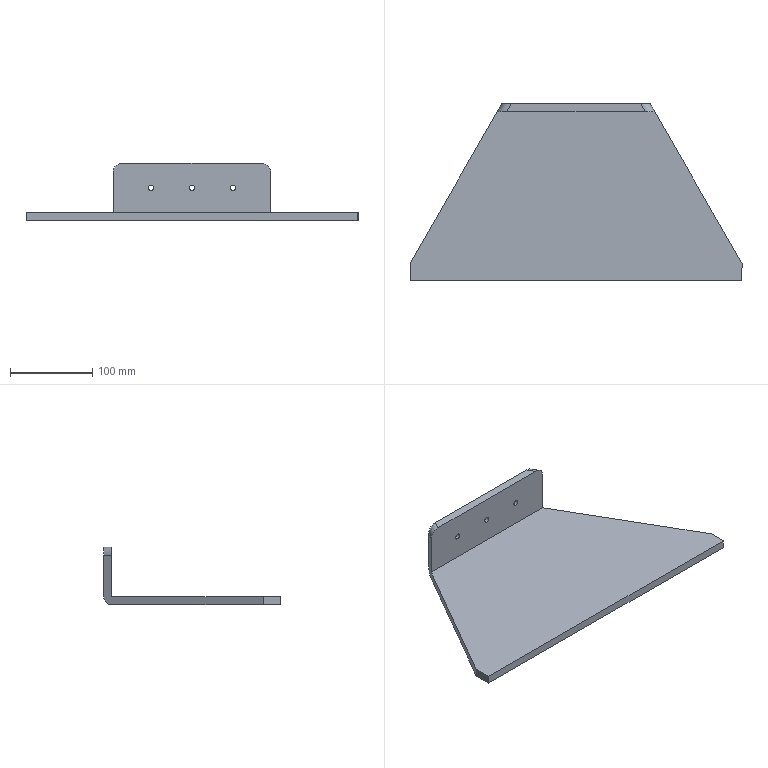Part | SolidWorks | features ICE 2, Extrusion 1, Fillet 1, HoleWzd 1, Shell 1 | 1 solid | 19 faces | box 404 x 215 x 70 mm | volume 757292 mm3 | plane 10 | cylinder 9 | commonest cylinder face diameters 6.8 x6 20 x3
STEP:
#1=CARTESIAN_POINT('',(-50.,97.5,43.4));
#2=VERTEX_POINT('',#1);
#3=CARTESIAN_POINT('',(-50.,97.5,36.6));
#4=VERTEX_POINT('',#3);
#5=CARTESIAN_POINT('',(-50.,97.5,40.));
#6=DIRECTION('',(0.,-1.,0.));
#7=DIRECTION('',(0.,0.,-1.));
#8=AXIS2_PLACEMENT_3D('',#5,#6,#7);
#9=CIRCLE('',#8,3.4);
#10=EDGE_CURVE('',#2,#4,#9,.T.);
#11=ORIENTED_EDGE('',*,*,#10,.T.);
#12=CARTESIAN_POINT('',(-50.,107.5,36.6));
#13=VERTEX_POINT('',#12);
#14=CARTESIAN_POINT('',(-50.,107.5,36.6));
#15=DIRECTION('',(0.,1.,0.));
#16=VECTOR('',#15,1000.);
#17=LINE('',#14,#16);
#18=EDGE_CURVE('',#4,#13,#17,.T.);
#19=ORIENTED_EDGE('',*,*,#18,.T.);
#20=CARTESIAN_POINT('',(-50.,107.5,43.4));
#21=VERTEX_POINT('',#20);
#22=CARTESIAN_POINT('',(-50.,107.5,40.));
#23=DIRECTION('',(0.,1.,0.));
#24=DIRECTION('',(0.,0.,1.));
#25=AXIS2_PLACEMENT_3D('',#22,#23,#24);
#26=CIRCLE('',#25,3.4);
#27=EDGE_CURVE('',#13,#21,#26,.T.);
#28=ORIENTED_EDGE('',*,*,#27,.T.);
#29=CARTESIAN_POINT('',(-50.,107.5,43.4));
#30=DIRECTION('',(0.,1.,0.));
#31=VECTOR('',#30,1000.);
#32=LINE('',#29,#31);
#33=EDGE_CURVE('',#2,#21,#32,.T.);
#34=ORIENTED_EDGE('',*,*,#33,.F.);
#35=EDGE_LOOP('',(#11,#19,#28,#34));
#36=FACE_OUTER_BOUND('',#35,.T.);
#37=CARTESIAN_POINT('',(-50.,107.5,40.));
#38=DIRECTION('',(0.,1.,0.));
#39=DIRECTION('',(0.,0.,1.));
#40=AXIS2_PLACEMENT_3D('',#37,#38,#39);
#41=CYLINDRICAL_SURFACE('',#40,3.4);
#42=ADVANCED_FACE('',(#36),#41,.F.);
#43=CARTESIAN_POINT('',(0.,97.5,43.4));
#44=VERTEX_POINT('',#43);
#45=CARTESIAN_POINT('',(0.,97.5,36.6));
#46=VERTEX_POINT('',#45);
#47=CARTESIAN_POINT('',(0.,97.5,40.));
#48=DIRECTION('',(0.,-1.,0.));
#49=DIRECTION('',(0.,0.,-1.));
#50=AXIS2_PLACEMENT_3D('',#47,#48,#49);
#51=CIRCLE('',#50,3.4);
#52=EDGE_CURVE('',#44,#46,#51,.T.);
#53=ORIENTED_EDGE('',*,*,#52,.T.);
#54=CARTESIAN_POINT('',(0.,107.5,36.6));
#55=VERTEX_POINT('',#54);
#56=CARTESIAN_POINT('',(0.,107.5,36.6));
#57=DIRECTION('',(0.,1.,0.));
#58=VECTOR('',#57,1000.);
#59=LINE('',#56,#58);
#60=EDGE_CURVE('',#46,#55,#59,.T.);
#61=ORIENTED_EDGE('',*,*,#60,.T.);
#62=CARTESIAN_POINT('',(0.,107.5,43.4));
#63=VERTEX_POINT('',#62);
#64=CARTESIAN_POINT('',(0.,107.5,40.));
#65=DIRECTION('',(0.,1.,0.));
#66=DIRECTION('',(0.,0.,1.));
#67=AXIS2_PLACEMENT_3D('',#64,#65,#66);
#68=CIRCLE('',#67,3.4);
#69=EDGE_CURVE('',#55,#63,#68,.T.);
#70=ORIENTED_EDGE('',*,*,#69,.T.);
#71=CARTESIAN_POINT('',(0.,107.5,43.4));
#72=DIRECTION('',(0.,1.,0.));
#73=VECTOR('',#72,1000.);
#74=LINE('',#71,#73);
#75=EDGE_CURVE('',#44,#63,#74,.T.);
#76=ORIENTED_EDGE('',*,*,#75,.F.);
#77=EDGE_LOOP('',(#53,#61,#70,#76));
#78=FACE_OUTER_BOUND('',#77,.T.);
#79=CARTESIAN_POINT('',(0.,107.5,40.));
#80=DIRECTION('',(0.,1.,0.));
#81=DIRECTION('',(0.,0.,1.));
#82=AXIS2_PLACEMENT_3D('',#79,#80,#81);
#83=CYLINDRICAL_SURFACE('',#82,3.4);
#84=ADVANCED_FACE('',(#78),#83,.F.);
#85=CARTESIAN_POINT('',(50.,97.5,43.4));
#86=VERTEX_POINT('',#85);
#87=CARTESIAN_POINT('',(50.,97.5,36.6));
#88=VERTEX_POINT('',#87);
#89=CARTESIAN_POINT('',(50.,97.5,40.));
#90=DIRECTION('',(0.,-1.,0.));
#91=DIRECTION('',(0.,0.,-1.));
#92=AXIS2_PLACEMENT_3D('',#89,#90,#91);
#93=CIRCLE('',#92,3.4);
#94=EDGE_CURVE('',#86,#88,#93,.T.);
#95=ORIENTED_EDGE('',*,*,#94,.T.);
#96=CARTESIAN_POINT('',(50.,107.5,36.6));
#97=VERTEX_POINT('',#96);
#98=CARTESIAN_POINT('',(50.,107.5,36.6));
#99=DIRECTION('',(0.,1.,0.));
#100=VECTOR('',#99,1000.);
#101=LINE('',#98,#100);
#102=EDGE_CURVE('',#88,#97,#101,.T.);
#103=ORIENTED_EDGE('',*,*,#102,.T.);
#104=CARTESIAN_POINT('',(50.,107.5,43.4));
#105=VERTEX_POINT('',#104);
#106=CARTESIAN_POINT('',(50.,107.5,40.));
#107=DIRECTION('',(0.,1.,0.));
#108=DIRECTION('',(0.,0.,1.));
#109=AXIS2_PLACEMENT_3D('',#106,#107,#108);
#110=CIRCLE('',#109,3.4);
#111=EDGE_CURVE('',#97,#105,#110,.T.);
#112=ORIENTED_EDGE('',*,*,#111,.T.);
#113=CARTESIAN_POINT('',(50.,107.5,43.4));
#114=DIRECTION('',(0.,1.,0.));
#115=VECTOR('',#114,1000.);
#116=LINE('',#113,#115);
#117=EDGE_CURVE('',#86,#105,#116,.T.);
#118=ORIENTED_EDGE('',*,*,#117,.F.);
#119=EDGE_LOOP('',(#95,#103,#112,#118));
#120=FACE_OUTER_BOUND('',#119,.T.);
#121=CARTESIAN_POINT('',(50.,107.5,40.));
#122=DIRECTION('',(0.,1.,0.));
#123=DIRECTION('',(0.,0.,1.));
#124=AXIS2_PLACEMENT_3D('',#121,#122,#123);
#125=CYLINDRICAL_SURFACE('',#124,3.4);
#126=ADVANCED_FACE('',(#120),#125,.F.);
#127=CARTESIAN_POINT('',(202.,-107.5,10.));
#128=VERTEX_POINT('',#127);
#129=CARTESIAN_POINT('',(202.,-86.49,10.));
#130=VERTEX_POINT('',#129);
#131=CARTESIAN_POINT('',(202.,107.5,10.));
#132=DIRECTION('',(0.,1.,0.));
#133=VECTOR('',#132,1000.);
#134=LINE('',#131,#133);
#135=EDGE_CURVE('',#128,#130,#134,.T.);
#136=ORIENTED_EDGE('',*,*,#135,.F.);
#137=CARTESIAN_POINT('',(202.,-107.5,0.));
#138=VERTEX_POINT('',#137);
#139=CARTESIAN_POINT('',(202.,-107.5,70.));
#140=DIRECTION('',(0.,0.,-1.));
#141=VECTOR('',#140,1000.);
#142=LINE('',#139,#141);
#143=EDGE_CURVE('',#128,#138,#142,.T.);
#144=ORIENTED_EDGE('',*,*,#143,.T.);
#145=CARTESIAN_POINT('',(202.,-86.49,0.));
#146=VERTEX_POINT('',#145);
#147=CARTESIAN_POINT('',(202.,107.5,0.));
#148=DIRECTION('',(0.,1.,0.));
#149=VECTOR('',#148,1000.);
#150=LINE('',#147,#149);
#151=EDGE_CURVE('',#138,#146,#150,.T.);
#152=ORIENTED_EDGE('',*,*,#151,.T.);
#153=CARTESIAN_POINT('',(202.,-86.49,-10.));
#154=DIRECTION('',(0.,0.,1.));
#155=VECTOR('',#154,1000.);
#156=LINE('',#153,#155);
#157=EDGE_CURVE('',#146,#130,#156,.T.);
#158=ORIENTED_EDGE('',*,*,#157,.T.);
#159=EDGE_LOOP('',(#136,#144,#152,#158));
#160=FACE_OUTER_BOUND('',#159,.T.);
#161=CARTESIAN_POINT('',(202.,107.5,70.));
#162=DIRECTION('',(-1.,0.,0.));
#163=DIRECTION('',(0.,-1.,0.));
#164=AXIS2_PLACEMENT_3D('',#161,#162,#163);
#165=PLANE('',#164);
#166=ADVANCED_FACE('',(#160),#165,.F.);
#167=CARTESIAN_POINT('',(-202.,-107.5,10.));
#168=VERTEX_POINT('',#167);
#169=CARTESIAN_POINT('',(-202.,-107.5,0.));
#170=VERTEX_POINT('',#169);
#171=CARTESIAN_POINT('',(-202.,-107.5,70.));
#172=DIRECTION('',(0.,0.,-1.));
#173=VECTOR('',#172,1000.);
#174=LINE('',#171,#173);
#175=EDGE_CURVE('',#168,#170,#174,.T.);
#176=ORIENTED_EDGE('',*,*,#175,.F.);
#177=CARTESIAN_POINT('',(-202.,-86.49,10.));
#178=VERTEX_POINT('',#177);
#179=CARTESIAN_POINT('',(-202.,107.5,10.));
#180=DIRECTION('',(0.,-1.,0.));
#181=VECTOR('',#180,1000.);
#182=LINE('',#179,#181);
#183=EDGE_CURVE('',#178,#168,#182,.T.);
#184=ORIENTED_EDGE('',*,*,#183,.F.);
#185=CARTESIAN_POINT('',(-202.,-86.49,0.));
#186=VERTEX_POINT('',#185);
#187=CARTESIAN_POINT('',(-202.,-86.49,-10.));
#188=DIRECTION('',(0.,0.,1.));
#189=VECTOR('',#188,1000.);
#190=LINE('',#187,#189);
#191=EDGE_CURVE('',#186,#178,#190,.T.);
#192=ORIENTED_EDGE('',*,*,#191,.F.);
#193=CARTESIAN_POINT('',(-202.,107.5,0.));
#194=DIRECTION('',(0.,-1.,0.));
#195=VECTOR('',#194,1000.);
#196=LINE('',#193,#195);
#197=EDGE_CURVE('',#186,#170,#196,.T.);
#198=ORIENTED_EDGE('',*,*,#197,.T.);
#199=EDGE_LOOP('',(#176,#184,#192,#198));
#200=FACE_OUTER_BOUND('',#199,.T.);
#201=CARTESIAN_POINT('',(-202.,107.5,70.));
#202=DIRECTION('',(1.,0.,0.));
#203=DIRECTION('',(0.,0.,-1.));
#204=AXIS2_PLACEMENT_3D('',#201,#202,#203);
#205=PLANE('',#204);
#206=ADVANCED_FACE('',(#200),#205,.F.);
#207=CARTESIAN_POINT('',(-50.,107.5,40.));
#208=DIRECTION('',(0.,1.,0.));
#209=DIRECTION('',(0.,0.,1.));
#210=AXIS2_PLACEMENT_3D('',#207,#208,#209);
#211=CIRCLE('',#210,3.4);
#212=EDGE_CURVE('',#21,#13,#211,.T.);
#213=ORIENTED_EDGE('',*,*,#212,.F.);
#214=ORIENTED_EDGE('',*,*,#27,.F.);
#215=EDGE_LOOP('',(#213,#214));
#216=FACE_BOUND('',#215,.T.);
#217=CARTESIAN_POINT('',(0.,107.5,40.));
#218=DIRECTION('',(0.,1.,0.));
#219=DIRECTION('',(0.,0.,1.));
#220=AXIS2_PLACEMENT_3D('',#217,#218,#219);
#221=CIRCLE('',#220,3.4);
#222=EDGE_CURVE('',#63,#55,#221,.T.);
#223=ORIENTED_EDGE('',*,*,#222,.F.);
#224=ORIENTED_EDGE('',*,*,#69,.F.);
#225=EDGE_LOOP('',(#223,#224));
#226=FACE_BOUND('',#225,.T.);
#227=CARTESIAN_POINT('',(50.,107.5,40.));
#228=DIRECTION('',(0.,1.,0.));
#229=DIRECTION('',(0.,0.,1.));
#230=AXIS2_PLACEMENT_3D('',#227,#228,#229);
#231=CIRCLE('',#230,3.4);
#232=EDGE_CURVE('',#105,#97,#231,.T.);
#233=ORIENTED_EDGE('',*,*,#232,.F.);
#234=ORIENTED_EDGE('',*,*,#111,.F.);
#235=EDGE_LOOP('',(#233,#234));
#236=FACE_BOUND('',#235,.T.);
#237=CARTESIAN_POINT('',(90.,107.5,10.));
#238=VERTEX_POINT('',#237);
#239=CARTESIAN_POINT('',(90.,107.5,60.));
#240=VERTEX_POINT('',#239);
#241=CARTESIAN_POINT('',(90.,107.5,-10.));
#242=DIRECTION('',(0.,0.,1.));
#243=VECTOR('',#242,1000.);
#244=LINE('',#241,#243);
#245=EDGE_CURVE('',#238,#240,#244,.T.);
#246=ORIENTED_EDGE('',*,*,#245,.F.);
#247=CARTESIAN_POINT('',(-90.,107.5,10.));
#248=VERTEX_POINT('',#247);
#249=CARTESIAN_POINT('',(-202.,107.5,10.));
#250=DIRECTION('',(-1.,0.,0.));
#251=VECTOR('',#250,1000.);
#252=LINE('',#249,#251);
#253=EDGE_CURVE('',#238,#248,#252,.T.);
#254=ORIENTED_EDGE('',*,*,#253,.T.);
#255=CARTESIAN_POINT('',(-90.,107.5,60.));
#256=VERTEX_POINT('',#255);
#257=CARTESIAN_POINT('',(-90.,107.5,-10.));
#258=DIRECTION('',(0.,0.,1.));
#259=VECTOR('',#258,1000.);
#260=LINE('',#257,#259);
#261=EDGE_CURVE('',#248,#256,#260,.T.);
#262=ORIENTED_EDGE('',*,*,#261,.T.);
#263=CARTESIAN_POINT('',(-78.453,107.5,70.));
#264=VERTEX_POINT('',#263);
#265=CARTESIAN_POINT('',(-90.,107.5,60.));
#266=CARTESIAN_POINT('',(-90.,107.5,65.858));
#267=CARTESIAN_POINT('',(-85.217,107.5,70.));
#268=CARTESIAN_POINT('',(-78.453,107.5,70.));
#269=(BOUNDED_CURVE()B_SPLINE_CURVE(3,(#265,#266,#267,#268),.UNSPECIFIED.,.F.,.F.)B_SPLINE_CURVE_WITH_KNOTS((4,4),(0.,1.571),.UNSPECIFIED.)CURVE()GEOMETRIC_REPRESENTATION_ITEM()RATIONAL_B_SPLINE_CURVE((1.,0.8047,0.8047,1.))REPRESENTATION_ITEM(''));
#270=EDGE_CURVE('',#256,#264,#269,.T.);
#271=ORIENTED_EDGE('',*,*,#270,.T.);
#272=CARTESIAN_POINT('',(78.453,107.5,70.));
#273=VERTEX_POINT('',#272);
#274=CARTESIAN_POINT('',(-202.,107.5,70.));
#275=DIRECTION('',(-1.,0.,0.));
#276=VECTOR('',#275,1000.);
#277=LINE('',#274,#276);
#278=EDGE_CURVE('',#273,#264,#277,.T.);
#279=ORIENTED_EDGE('',*,*,#278,.F.);
#280=CARTESIAN_POINT('',(78.453,107.5,70.));
#281=CARTESIAN_POINT('',(85.217,107.5,70.));
#282=CARTESIAN_POINT('',(90.,107.5,65.858));
#283=CARTESIAN_POINT('',(90.,107.5,60.));
#284=(BOUNDED_CURVE()B_SPLINE_CURVE(3,(#280,#281,#282,#283),.UNSPECIFIED.,.F.,.F.)B_SPLINE_CURVE_WITH_KNOTS((4,4),(1.571,3.142),.UNSPECIFIED.)CURVE()GEOMETRIC_REPRESENTATION_ITEM()RATIONAL_B_SPLINE_CURVE((1.,0.8047,0.8047,1.))REPRESENTATION_ITEM(''));
#285=EDGE_CURVE('',#273,#240,#284,.T.);
#286=ORIENTED_EDGE('',*,*,#285,.T.);
#287=EDGE_LOOP('',(#246,#254,#262,#271,#279,#286));
#288=FACE_OUTER_BOUND('',#287,.T.);
#289=CARTESIAN_POINT('',(-202.,107.5,70.));
#290=DIRECTION('',(0.,-1.,0.));
#291=DIRECTION('',(0.,0.,-1.));
#292=AXIS2_PLACEMENT_3D('',#289,#290,#291);
#293=PLANE('',#292);
#294=ADVANCED_FACE('',(#216,#226,#236,#288),#293,.F.);
#295=ORIENTED_EDGE('',*,*,#143,.F.);
#296=CARTESIAN_POINT('',(-642.963,-107.5,10.));
#297=DIRECTION('',(1.,0.,0.));
#298=VECTOR('',#297,1000.);
#299=LINE('',#296,#298);
#300=EDGE_CURVE('',#168,#128,#299,.T.);
#301=ORIENTED_EDGE('',*,*,#300,.F.);
#302=ORIENTED_EDGE('',*,*,#175,.T.);
#303=CARTESIAN_POINT('',(-202.,-107.5,0.));
#304=DIRECTION('',(1.,0.,0.));
#305=VECTOR('',#304,1000.);
#306=LINE('',#303,#305);
#307=EDGE_CURVE('',#170,#138,#306,.T.);
#308=ORIENTED_EDGE('',*,*,#307,.T.);
#309=EDGE_LOOP('',(#295,#301,#302,#308));
#310=FACE_OUTER_BOUND('',#309,.T.);
#311=CARTESIAN_POINT('',(-202.,-107.5,70.));
#312=DIRECTION('',(0.,1.,0.));
#313=DIRECTION('',(0.,0.,1.));
#314=AXIS2_PLACEMENT_3D('',#311,#312,#313);
#315=PLANE('',#314);
#316=ADVANCED_FACE('',(#310),#315,.F.);
#317=CARTESIAN_POINT('',(84.226,97.5,70.));
#318=VERTEX_POINT('',#317);
#319=CARTESIAN_POINT('',(-84.226,97.5,70.));
#320=VERTEX_POINT('',#319);
#321=CARTESIAN_POINT('',(0.,97.5,70.));
#322=DIRECTION('',(-1.,0.,0.));
#323=VECTOR('',#322,1000.);
#324=LINE('',#321,#323);
#325=EDGE_CURVE('',#318,#320,#324,.T.);
#326=ORIENTED_EDGE('',*,*,#325,.F.);
#327=CARTESIAN_POINT('',(81.34,102.5,70.));
#328=DIRECTION('',(-0.5,0.866,0.));
#329=VECTOR('',#328,1000.);
#330=LINE('',#327,#329);
#331=EDGE_CURVE('',#318,#273,#330,.T.);
#332=ORIENTED_EDGE('',*,*,#331,.T.);
#333=ORIENTED_EDGE('',*,*,#278,.T.);
#334=CARTESIAN_POINT('',(-87.113,92.5,70.));
#335=DIRECTION('',(-0.5,-0.866,0.));
#336=VECTOR('',#335,1000.);
#337=LINE('',#334,#336);
#338=EDGE_CURVE('',#264,#320,#337,.T.);
#339=ORIENTED_EDGE('',*,*,#338,.T.);
#340=EDGE_LOOP('',(#326,#332,#333,#339));
#341=FACE_OUTER_BOUND('',#340,.T.);
#342=CARTESIAN_POINT('',(0.,0.,70.));
#343=DIRECTION('',(0.,0.,1.));
#344=DIRECTION('',(1.,0.,0.));
#345=AXIS2_PLACEMENT_3D('',#342,#343,#344);
#346=PLANE('',#345);
#347=ADVANCED_FACE('',(#341),#346,.T.);
#348=CARTESIAN_POINT('',(-95.774,97.5,0.));
#349=VERTEX_POINT('',#348);
#350=CARTESIAN_POINT('',(-114.049,65.846,0.));
#351=DIRECTION('',(0.5,0.866,0.));
#352=VECTOR('',#351,1000.);
#353=LINE('',#350,#352);
#354=EDGE_CURVE('',#186,#349,#353,.T.);
#355=ORIENTED_EDGE('',*,*,#354,.T.);
#356=CARTESIAN_POINT('',(95.774,97.5,0.));
#357=VERTEX_POINT('',#356);
#358=CARTESIAN_POINT('',(0.,97.5,0.));
#359=DIRECTION('',(1.,0.,0.));
#360=VECTOR('',#359,1000.);
#361=LINE('',#358,#360);
#362=EDGE_CURVE('',#349,#357,#361,.T.);
#363=ORIENTED_EDGE('',*,*,#362,.T.);
#364=CARTESIAN_POINT('',(114.049,65.846,0.));
#365=DIRECTION('',(0.5,-0.866,0.));
#366=VECTOR('',#365,1000.);
#367=LINE('',#364,#366);
#368=EDGE_CURVE('',#357,#146,#367,.T.);
#369=ORIENTED_EDGE('',*,*,#368,.T.);
#370=ORIENTED_EDGE('',*,*,#151,.F.);
#371=ORIENTED_EDGE('',*,*,#307,.F.);
#372=ORIENTED_EDGE('',*,*,#197,.F.);
#373=EDGE_LOOP('',(#355,#363,#369,#370,#371,#372));
#374=FACE_OUTER_BOUND('',#373,.T.);
#375=CARTESIAN_POINT('',(0.,0.,0.));
#376=DIRECTION('',(0.,0.,1.));
#377=DIRECTION('',(1.,0.,0.));
#378=AXIS2_PLACEMENT_3D('',#375,#376,#377);
#379=PLANE('',#378);
#380=ADVANCED_FACE('',(#374),#379,.F.);
#381=ORIENTED_EDGE('',*,*,#10,.F.);
#382=CARTESIAN_POINT('',(-50.,97.5,40.));
#383=DIRECTION('',(0.,-1.,0.));
#384=DIRECTION('',(0.,0.,-1.));
#385=AXIS2_PLACEMENT_3D('',#382,#383,#384);
#386=CIRCLE('',#385,3.4);
#387=EDGE_CURVE('',#4,#2,#386,.T.);
#388=ORIENTED_EDGE('',*,*,#387,.F.);
#389=EDGE_LOOP('',(#381,#388));
#390=FACE_BOUND('',#389,.T.);
#391=ORIENTED_EDGE('',*,*,#52,.F.);
#392=CARTESIAN_POINT('',(0.,97.5,40.));
#393=DIRECTION('',(0.,-1.,0.));
#394=DIRECTION('',(0.,0.,-1.));
#395=AXIS2_PLACEMENT_3D('',#392,#393,#394);
#396=CIRCLE('',#395,3.4);
#397=EDGE_CURVE('',#46,#44,#396,.T.);
#398=ORIENTED_EDGE('',*,*,#397,.F.);
#399=EDGE_LOOP('',(#391,#398));
#400=FACE_BOUND('',#399,.T.);
#401=ORIENTED_EDGE('',*,*,#94,.F.);
#402=CARTESIAN_POINT('',(50.,97.5,40.));
#403=DIRECTION('',(0.,-1.,0.));
#404=DIRECTION('',(0.,0.,-1.));
#405=AXIS2_PLACEMENT_3D('',#402,#403,#404);
#406=CIRCLE('',#405,3.4);
#407=EDGE_CURVE('',#88,#86,#406,.T.);
#408=ORIENTED_EDGE('',*,*,#407,.F.);
#409=EDGE_LOOP('',(#401,#408));
#410=FACE_BOUND('',#409,.T.);
#411=CARTESIAN_POINT('',(95.774,97.5,60.));
#412=VERTEX_POINT('',#411);
#413=CARTESIAN_POINT('',(95.774,97.5,10.));
#414=VERTEX_POINT('',#413);
#415=CARTESIAN_POINT('',(95.774,97.5,70.));
#416=DIRECTION('',(0.,0.,-1.));
#417=VECTOR('',#416,1000.);
#418=LINE('',#415,#417);
#419=EDGE_CURVE('',#412,#414,#418,.T.);
#420=ORIENTED_EDGE('',*,*,#419,.F.);
#421=CARTESIAN_POINT('',(95.774,97.5,60.));
#422=CARTESIAN_POINT('',(95.774,97.5,65.858));
#423=CARTESIAN_POINT('',(90.991,97.5,70.));
#424=CARTESIAN_POINT('',(84.226,97.5,70.));
#425=(BOUNDED_CURVE()B_SPLINE_CURVE(3,(#421,#422,#423,#424),.UNSPECIFIED.,.F.,.F.)B_SPLINE_CURVE_WITH_KNOTS((4,4),(3.142,4.712),.UNSPECIFIED.)CURVE()GEOMETRIC_REPRESENTATION_ITEM()RATIONAL_B_SPLINE_CURVE((1.,0.8047,0.8047,1.))REPRESENTATION_ITEM(''));
#426=EDGE_CURVE('',#412,#318,#425,.T.);
#427=ORIENTED_EDGE('',*,*,#426,.T.);
#428=ORIENTED_EDGE('',*,*,#325,.T.);
#429=CARTESIAN_POINT('',(-95.774,97.5,60.));
#430=VERTEX_POINT('',#429);
#431=CARTESIAN_POINT('',(-84.226,97.5,70.));
#432=CARTESIAN_POINT('',(-90.991,97.5,70.));
#433=CARTESIAN_POINT('',(-95.774,97.5,65.858));
#434=CARTESIAN_POINT('',(-95.774,97.5,60.));
#435=(BOUNDED_CURVE()B_SPLINE_CURVE(3,(#431,#432,#433,#434),.UNSPECIFIED.,.F.,.F.)B_SPLINE_CURVE_WITH_KNOTS((4,4),(4.712,6.283),.UNSPECIFIED.)CURVE()GEOMETRIC_REPRESENTATION_ITEM()RATIONAL_B_SPLINE_CURVE((1.,0.8047,0.8047,1.))REPRESENTATION_ITEM(''));
#436=EDGE_CURVE('',#320,#430,#435,.T.);
#437=ORIENTED_EDGE('',*,*,#436,.T.);
#438=CARTESIAN_POINT('',(-95.774,97.5,10.));
#439=VERTEX_POINT('',#438);
#440=CARTESIAN_POINT('',(-95.774,97.5,70.));
#441=DIRECTION('',(0.,0.,1.));
#442=VECTOR('',#441,1000.);
#443=LINE('',#440,#442);
#444=EDGE_CURVE('',#439,#430,#443,.T.);
#445=ORIENTED_EDGE('',*,*,#444,.F.);
#446=CARTESIAN_POINT('',(-202.,97.5,10.));
#447=DIRECTION('',(-1.,0.,0.));
#448=VECTOR('',#447,1000.);
#449=LINE('',#446,#448);
#450=EDGE_CURVE('',#414,#439,#449,.T.);
#451=ORIENTED_EDGE('',*,*,#450,.F.);
#452=EDGE_LOOP('',(#420,#427,#428,#437,#445,#451));
#453=FACE_OUTER_BOUND('',#452,.T.);
#454=CARTESIAN_POINT('',(-202.,97.5,70.));
#455=DIRECTION('',(0.,-1.,0.));
#456=DIRECTION('',(0.,0.,-1.));
#457=AXIS2_PLACEMENT_3D('',#454,#455,#456);
#458=PLANE('',#457);
#459=ADVANCED_FACE('',(#390,#400,#410,#453),#458,.T.);
#460=CARTESIAN_POINT('',(-114.049,65.846,10.));
#461=DIRECTION('',(0.5,0.866,0.));
#462=VECTOR('',#461,1000.);
#463=LINE('',#460,#462);
#464=EDGE_CURVE('',#178,#439,#463,.T.);
#465=ORIENTED_EDGE('',*,*,#464,.F.);
#466=ORIENTED_EDGE('',*,*,#183,.T.);
#467=ORIENTED_EDGE('',*,*,#300,.T.);
#468=ORIENTED_EDGE('',*,*,#135,.T.);
#469=CARTESIAN_POINT('',(114.049,65.846,10.));
#470=DIRECTION('',(0.5,-0.866,0.));
#471=VECTOR('',#470,1000.);
#472=LINE('',#469,#471);
#473=EDGE_CURVE('',#414,#130,#472,.T.);
#474=ORIENTED_EDGE('',*,*,#473,.F.);
#475=ORIENTED_EDGE('',*,*,#450,.T.);
#476=EDGE_LOOP('',(#465,#466,#467,#468,#474,#475));
#477=FACE_OUTER_BOUND('',#476,.T.);
#478=CARTESIAN_POINT('',(0.,0.,10.));
#479=DIRECTION('',(0.,0.,1.));
#480=DIRECTION('',(1.,0.,0.));
#481=AXIS2_PLACEMENT_3D('',#478,#479,#480);
#482=PLANE('',#481);
#483=ADVANCED_FACE('',(#477),#482,.T.);
#484=ORIENTED_EDGE('',*,*,#368,.F.);
#485=CARTESIAN_POINT('',(95.774,97.5,0.));
#486=CARTESIAN_POINT('',(92.391,103.358,0.));
#487=CARTESIAN_POINT('',(90.,107.5,4.142));
#488=CARTESIAN_POINT('',(90.,107.5,10.));
#489=(BOUNDED_CURVE()B_SPLINE_CURVE(3,(#485,#486,#487,#488),.UNSPECIFIED.,.F.,.T.)B_SPLINE_CURVE_WITH_KNOTS((4,4),(4.712,6.283),.UNSPECIFIED.)CURVE()GEOMETRIC_REPRESENTATION_ITEM()RATIONAL_B_SPLINE_CURVE((1.,0.8047,0.8047,1.))REPRESENTATION_ITEM(''));
#490=EDGE_CURVE('',#357,#238,#489,.T.);
#491=ORIENTED_EDGE('',*,*,#490,.T.);
#492=ORIENTED_EDGE('',*,*,#245,.T.);
#493=CARTESIAN_POINT('',(95.774,97.5,60.));
#494=DIRECTION('',(0.5,-0.866,0.));
#495=VECTOR('',#494,1000.);
#496=LINE('',#493,#495);
#497=EDGE_CURVE('',#240,#412,#496,.T.);
#498=ORIENTED_EDGE('',*,*,#497,.T.);
#499=ORIENTED_EDGE('',*,*,#419,.T.);
#500=ORIENTED_EDGE('',*,*,#473,.T.);
#501=ORIENTED_EDGE('',*,*,#157,.F.);
#502=EDGE_LOOP('',(#484,#491,#492,#498,#499,#500,#501));
#503=FACE_OUTER_BOUND('',#502,.T.);
#504=CARTESIAN_POINT('',(202.,-86.49,-10.));
#505=DIRECTION('',(-0.866,-0.5,0.));
#506=DIRECTION('',(0.5,-0.866,0.));
#507=AXIS2_PLACEMENT_3D('',#504,#505,#506);
#508=PLANE('',#507);
#509=ADVANCED_FACE('',(#503),#508,.F.);
#510=ORIENTED_EDGE('',*,*,#261,.F.);
#511=CARTESIAN_POINT('',(-90.,107.5,10.));
#512=CARTESIAN_POINT('',(-90.,107.5,4.142));
#513=CARTESIAN_POINT('',(-92.391,103.358,0.));
#514=CARTESIAN_POINT('',(-95.774,97.5,0.));
#515=(BOUNDED_CURVE()B_SPLINE_CURVE(3,(#511,#512,#513,#514),.UNSPECIFIED.,.F.,.T.)B_SPLINE_CURVE_WITH_KNOTS((4,4),(3.142,4.712),.UNSPECIFIED.)CURVE()GEOMETRIC_REPRESENTATION_ITEM()RATIONAL_B_SPLINE_CURVE((1.,0.8047,0.8047,1.))REPRESENTATION_ITEM(''));
#516=EDGE_CURVE('',#248,#349,#515,.T.);
#517=ORIENTED_EDGE('',*,*,#516,.T.);
#518=ORIENTED_EDGE('',*,*,#354,.F.);
#519=ORIENTED_EDGE('',*,*,#191,.T.);
#520=ORIENTED_EDGE('',*,*,#464,.T.);
#521=ORIENTED_EDGE('',*,*,#444,.T.);
#522=CARTESIAN_POINT('',(-90.,107.5,60.));
#523=DIRECTION('',(0.5,0.866,0.));
#524=VECTOR('',#523,1000.);
#525=LINE('',#522,#524);
#526=EDGE_CURVE('',#430,#256,#525,.T.);
#527=ORIENTED_EDGE('',*,*,#526,.T.);
#528=EDGE_LOOP('',(#510,#517,#518,#519,#520,#521,#527));
#529=FACE_OUTER_BOUND('',#528,.T.);
#530=CARTESIAN_POINT('',(-202.,-86.49,-10.));
#531=DIRECTION('',(0.866,-0.5,0.));
#532=DIRECTION('',(0.5,0.866,0.));
#533=AXIS2_PLACEMENT_3D('',#530,#531,#532);
#534=PLANE('',#533);
#535=ADVANCED_FACE('',(#529),#534,.F.);
#536=ORIENTED_EDGE('',*,*,#102,.F.);
#537=ORIENTED_EDGE('',*,*,#407,.T.);
#538=ORIENTED_EDGE('',*,*,#117,.T.);
#539=ORIENTED_EDGE('',*,*,#232,.T.);
#540=EDGE_LOOP('',(#536,#537,#538,#539));
#541=FACE_OUTER_BOUND('',#540,.T.);
#542=CARTESIAN_POINT('',(50.,107.5,40.));
#543=DIRECTION('',(0.,1.,0.));
#544=DIRECTION('',(0.,0.,1.));
#545=AXIS2_PLACEMENT_3D('',#542,#543,#544);
#546=CYLINDRICAL_SURFACE('',#545,3.4);
#547=ADVANCED_FACE('',(#541),#546,.F.);
#548=ORIENTED_EDGE('',*,*,#60,.F.);
#549=ORIENTED_EDGE('',*,*,#397,.T.);
#550=ORIENTED_EDGE('',*,*,#75,.T.);
#551=ORIENTED_EDGE('',*,*,#222,.T.);
#552=EDGE_LOOP('',(#548,#549,#550,#551));
#553=FACE_OUTER_BOUND('',#552,.T.);
#554=CARTESIAN_POINT('',(0.,107.5,40.));
#555=DIRECTION('',(0.,1.,0.));
#556=DIRECTION('',(0.,0.,1.));
#557=AXIS2_PLACEMENT_3D('',#554,#555,#556);
#558=CYLINDRICAL_SURFACE('',#557,3.4);
#559=ADVANCED_FACE('',(#553),#558,.F.);
#560=ORIENTED_EDGE('',*,*,#18,.F.);
#561=ORIENTED_EDGE('',*,*,#387,.T.);
#562=ORIENTED_EDGE('',*,*,#33,.T.);
#563=ORIENTED_EDGE('',*,*,#212,.T.);
#564=EDGE_LOOP('',(#560,#561,#562,#563));
#565=FACE_OUTER_BOUND('',#564,.T.);
#566=CARTESIAN_POINT('',(-50.,107.5,40.));
#567=DIRECTION('',(0.,1.,0.));
#568=DIRECTION('',(0.,0.,1.));
#569=AXIS2_PLACEMENT_3D('',#566,#567,#568);
#570=CYLINDRICAL_SURFACE('',#569,3.4);
#571=ADVANCED_FACE('',(#565),#570,.F.);
#572=ORIENTED_EDGE('',*,*,#490,.F.);
#573=ORIENTED_EDGE('',*,*,#362,.F.);
#574=ORIENTED_EDGE('',*,*,#516,.F.);
#575=ORIENTED_EDGE('',*,*,#253,.F.);
#576=EDGE_LOOP('',(#572,#573,#574,#575));
#577=FACE_OUTER_BOUND('',#576,.T.);
#578=CARTESIAN_POINT('',(-202.,97.5,10.));
#579=DIRECTION('',(-1.,0.,0.));
#580=DIRECTION('',(0.,0.,1.));
#581=AXIS2_PLACEMENT_3D('',#578,#579,#580);
#582=CYLINDRICAL_SURFACE('',#581,10.);
#583=ADVANCED_FACE('',(#577),#582,.T.);
#584=ORIENTED_EDGE('',*,*,#285,.F.);
#585=ORIENTED_EDGE('',*,*,#331,.F.);
#586=ORIENTED_EDGE('',*,*,#426,.F.);
#587=ORIENTED_EDGE('',*,*,#497,.F.);
#588=EDGE_LOOP('',(#584,#585,#586,#587));
#589=FACE_OUTER_BOUND('',#588,.T.);
#590=CARTESIAN_POINT('',(193.34,-91.49,60.));
#591=DIRECTION('',(-0.5,0.866,0.));
#592=DIRECTION('',(-0.866,-0.5,0.));
#593=AXIS2_PLACEMENT_3D('',#590,#591,#592);
#594=CYLINDRICAL_SURFACE('',#593,10.);
#595=ADVANCED_FACE('',(#589),#594,.T.);
#596=ORIENTED_EDGE('',*,*,#436,.F.);
#597=ORIENTED_EDGE('',*,*,#338,.F.);
#598=ORIENTED_EDGE('',*,*,#270,.F.);
#599=ORIENTED_EDGE('',*,*,#526,.F.);
#600=EDGE_LOOP('',(#596,#597,#598,#599));
#601=FACE_OUTER_BOUND('',#600,.T.);
#602=CARTESIAN_POINT('',(-193.34,-91.49,60.));
#603=DIRECTION('',(-0.5,-0.866,0.));
#604=DIRECTION('',(0.866,-0.5,0.));
#605=AXIS2_PLACEMENT_3D('',#602,#603,#604);
#606=CYLINDRICAL_SURFACE('',#605,10.);
#607=ADVANCED_FACE('',(#601),#606,.T.);
#608=CLOSED_SHELL('',(#42,#84,#126,#166,#206,#294,#316,#347,#380,#459,#483,#509,#535,#547,#559,#571,#583,#595,#607));
#609=MANIFOLD_SOLID_BREP('',#608);
#610=CARTESIAN_POINT('',(0.,0.,0.));
#611=DIRECTION('',(0.,0.,1.));
#612=DIRECTION('',(1.,0.,0.));
#613=AXIS2_PLACEMENT_3D('',#610,#611,#612);
#614=(LENGTH_UNIT()NAMED_UNIT(*)SI_UNIT(.MILLI.,.METRE.));
#615=UNCERTAINTY_MEASURE_WITH_UNIT(LENGTH_MEASURE(0.00001),#614,'','');
#616=(NAMED_UNIT(*)PLANE_ANGLE_UNIT()SI_UNIT($,.RADIAN.));
#617=(NAMED_UNIT(*)SI_UNIT($,.STERADIAN.)SOLID_ANGLE_UNIT());
#618=(GEOMETRIC_REPRESENTATION_CONTEXT(3)GLOBAL_UNCERTAINTY_ASSIGNED_CONTEXT((#615))GLOBAL_UNIT_ASSIGNED_CONTEXT((#614,#616,#617))REPRESENTATION_CONTEXT('',''));
#619=ADVANCED_BREP_SHAPE_REPRESENTATION('',(#609,#613),#618);